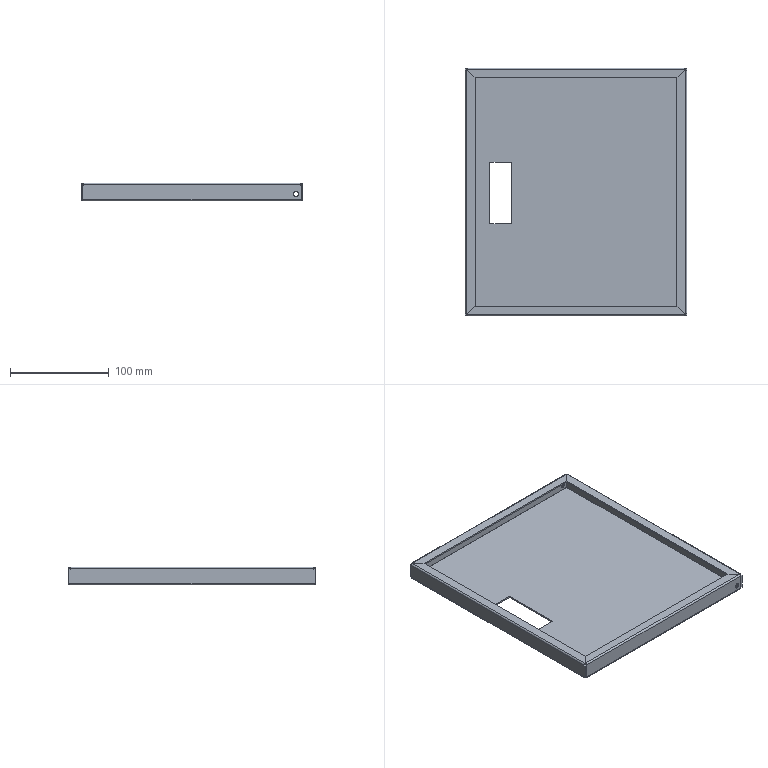Part | 1 solid | 126 faces | box 224.5 x 251 x 18 mm | volume 116249 mm3 | plane 106 | cylinder 20 | commonest cylinder face diameters 0.2 x8 3.2 x8 5.2 x4